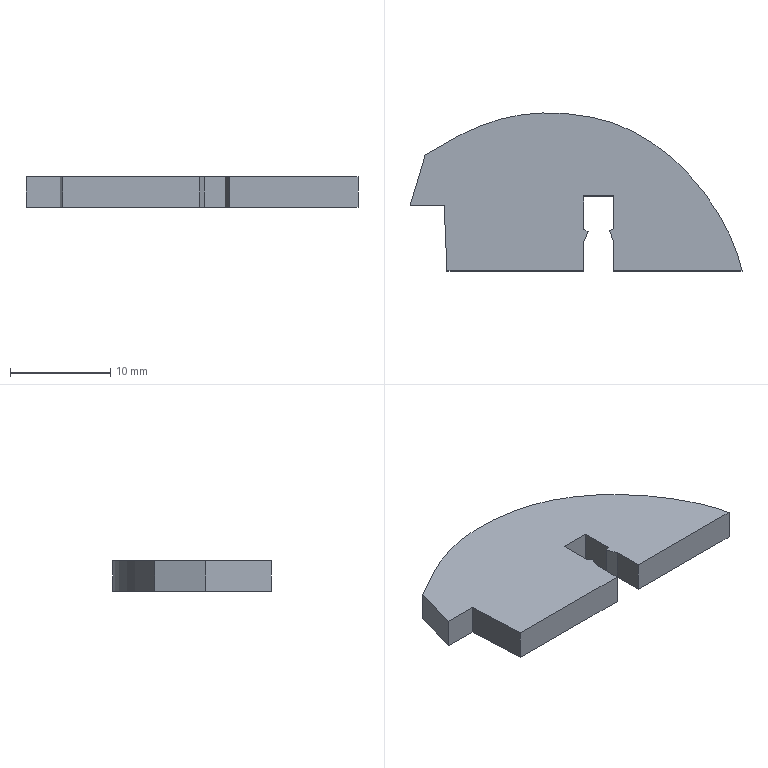Part | SolidWorks | features BaseBody 1 | 1 solid | 18 faces | box 33.145 x 15.784 x 3 mm | volume 1116 mm3 | plane 15 | spline 3
STEP:
#1=CARTESIAN_POINT('',(-1.198,15.692,-1.5));
#2=VERTEX_POINT('',#1);
#3=CARTESIAN_POINT('',(13.751,0.3596,-1.5));
#4=VERTEX_POINT('',#3);
#5=CARTESIAN_POINT('',(-1.198,15.692,-1.5));
#6=CARTESIAN_POINT('',(7.041,14.092,-1.5));
#7=CARTESIAN_POINT('',(12.666,5.726,-1.5));
#8=CARTESIAN_POINT('',(13.751,0.3596,-1.5));
#9=B_SPLINE_CURVE_WITH_KNOTS('',3,(#5,#6,#7,#8),.UNSPECIFIED.,.F.,.F.,(4,4),(0.3636,0.4545),.UNSPECIFIED.);
#10=EDGE_CURVE('',#2,#4,#9,.T.);
#11=ORIENTED_EDGE('',*,*,#10,.T.);
#12=CARTESIAN_POINT('',(0.9453,0.3596,-1.5));
#13=VERTEX_POINT('',#12);
#14=CARTESIAN_POINT('',(0.,0.3596,-1.5));
#15=DIRECTION('',(-1.,0.,0.));
#16=VECTOR('',#15,1000.);
#17=LINE('',#14,#16);
#18=EDGE_CURVE('',#4,#13,#17,.T.);
#19=ORIENTED_EDGE('',*,*,#18,.T.);
#20=CARTESIAN_POINT('',(0.9453,3.34,-1.5));
#21=VERTEX_POINT('',#20);
#22=CARTESIAN_POINT('',(0.9453,0.,-1.5));
#23=DIRECTION('',(0.,-1.,0.));
#24=VECTOR('',#23,1000.);
#25=LINE('',#22,#24);
#26=EDGE_CURVE('',#21,#13,#25,.T.);
#27=ORIENTED_EDGE('',*,*,#26,.F.);
#28=CARTESIAN_POINT('',(0.4951,4.381,-1.5));
#29=VERTEX_POINT('',#28);
#30=CARTESIAN_POINT('',(2.013,0.8704,-1.5));
#31=DIRECTION('',(0.3969,-0.9179,0.));
#32=VECTOR('',#31,1000.);
#33=LINE('',#30,#32);
#34=EDGE_CURVE('',#29,#21,#33,.T.);
#35=ORIENTED_EDGE('',*,*,#34,.F.);
#36=CARTESIAN_POINT('',(0.9453,4.577,-1.5));
#37=VERTEX_POINT('',#36);
#38=CARTESIAN_POINT('',(-1.524,3.502,-1.5));
#39=DIRECTION('',(-0.9169,-0.3992,0.));
#40=VECTOR('',#39,1000.);
#41=LINE('',#38,#40);
#42=EDGE_CURVE('',#37,#29,#41,.T.);
#43=ORIENTED_EDGE('',*,*,#42,.F.);
#44=CARTESIAN_POINT('',(0.9453,7.848,-1.5));
#45=VERTEX_POINT('',#44);
#46=CARTESIAN_POINT('',(0.9453,0.,-1.5));
#47=DIRECTION('',(0.,-1.,0.));
#48=VECTOR('',#47,1000.);
#49=LINE('',#46,#48);
#50=EDGE_CURVE('',#45,#37,#49,.T.);
#51=ORIENTED_EDGE('',*,*,#50,.F.);
#52=CARTESIAN_POINT('',(-2.051,7.848,-1.5));
#53=VERTEX_POINT('',#52);
#54=CARTESIAN_POINT('',(0.,7.848,-1.5));
#55=DIRECTION('',(1.,0.,0.));
#56=VECTOR('',#55,1000.);
#57=LINE('',#54,#56);
#58=EDGE_CURVE('',#53,#45,#57,.T.);
#59=ORIENTED_EDGE('',*,*,#58,.F.);
#60=CARTESIAN_POINT('',(-2.051,4.544,-1.5));
#61=VERTEX_POINT('',#60);
#62=CARTESIAN_POINT('',(-2.051,0.,-1.5));
#63=DIRECTION('',(0.,1.,0.));
#64=VECTOR('',#63,1000.);
#65=LINE('',#62,#64);
#66=EDGE_CURVE('',#61,#53,#65,.T.);
#67=ORIENTED_EDGE('',*,*,#66,.F.);
#68=CARTESIAN_POINT('',(-1.602,4.279,-1.5));
#69=VERTEX_POINT('',#68);
#70=CARTESIAN_POINT('',(1.459,2.47,-1.5));
#71=DIRECTION('',(-0.861,0.5086,0.));
#72=VECTOR('',#71,1000.);
#73=LINE('',#70,#72);
#74=EDGE_CURVE('',#69,#61,#73,.T.);
#75=ORIENTED_EDGE('',*,*,#74,.F.);
#76=CARTESIAN_POINT('',(-2.051,3.321,-1.5));
#77=VERTEX_POINT('',#76);
#78=CARTESIAN_POINT('',(-2.957,1.385,-1.5));
#79=DIRECTION('',(0.4242,0.9056,0.));
#80=VECTOR('',#79,1000.);
#81=LINE('',#78,#80);
#82=EDGE_CURVE('',#77,#69,#81,.T.);
#83=ORIENTED_EDGE('',*,*,#82,.F.);
#84=CARTESIAN_POINT('',(-2.051,0.3596,-1.5));
#85=VERTEX_POINT('',#84);
#86=CARTESIAN_POINT('',(-2.051,0.,-1.5));
#87=DIRECTION('',(0.,1.,0.));
#88=VECTOR('',#87,1000.);
#89=LINE('',#86,#88);
#90=EDGE_CURVE('',#85,#77,#89,.T.);
#91=ORIENTED_EDGE('',*,*,#90,.F.);
#92=CARTESIAN_POINT('',(-15.701,0.3596,-1.5));
#93=VERTEX_POINT('',#92);
#94=CARTESIAN_POINT('',(0.,0.3596,-1.5));
#95=DIRECTION('',(-1.,0.,0.));
#96=VECTOR('',#95,1000.);
#97=LINE('',#94,#96);
#98=EDGE_CURVE('',#85,#93,#97,.T.);
#99=ORIENTED_EDGE('',*,*,#98,.T.);
#100=CARTESIAN_POINT('',(-15.986,6.867,-1.5));
#101=VERTEX_POINT('',#100);
#102=CARTESIAN_POINT('',(-15.701,0.3596,-1.5));
#103=CARTESIAN_POINT('',(-15.797,2.531,-1.5));
#104=CARTESIAN_POINT('',(-15.89,4.698,-1.5));
#105=CARTESIAN_POINT('',(-15.986,6.867,-1.5));
#106=B_SPLINE_CURVE_WITH_KNOTS('',3,(#102,#103,#104,#105),.UNSPECIFIED.,.F.,.F.,(4,4),(0.,0.09091),.UNSPECIFIED.);
#107=EDGE_CURVE('',#93,#101,#106,.T.);
#108=ORIENTED_EDGE('',*,*,#107,.T.);
#109=CARTESIAN_POINT('',(-19.394,6.867,-1.5));
#110=VERTEX_POINT('',#109);
#111=CARTESIAN_POINT('',(0.,6.867,-1.5));
#112=DIRECTION('',(-1.,0.,0.));
#113=VECTOR('',#112,1000.);
#114=LINE('',#111,#113);
#115=EDGE_CURVE('',#101,#110,#114,.T.);
#116=ORIENTED_EDGE('',*,*,#115,.T.);
#117=CARTESIAN_POINT('',(-17.871,11.949,-1.5));
#118=VERTEX_POINT('',#117);
#119=CARTESIAN_POINT('',(-19.684,5.899,-1.5));
#120=DIRECTION('',(0.2871,0.9579,0.));
#121=VECTOR('',#120,1000.);
#122=LINE('',#119,#121);
#123=EDGE_CURVE('',#110,#118,#122,.T.);
#124=ORIENTED_EDGE('',*,*,#123,.T.);
#125=CARTESIAN_POINT('',(-17.871,11.949,-1.5));
#126=CARTESIAN_POINT('',(-13.479,14.586,-1.5));
#127=CARTESIAN_POINT('',(-9.088,17.223,-1.5));
#128=CARTESIAN_POINT('',(-1.198,15.692,-1.5));
#129=B_SPLINE_CURVE_WITH_KNOTS('',3,(#125,#126,#127,#128),.UNSPECIFIED.,.F.,.F.,(4,4),(0.2727,0.3636),.UNSPECIFIED.);
#130=EDGE_CURVE('',#118,#2,#129,.T.);
#131=ORIENTED_EDGE('',*,*,#130,.T.);
#132=EDGE_LOOP('',(#11,#19,#27,#35,#43,#51,#59,#67,#75,#83,#91,#99,#108,#116,#124,#131));
#133=FACE_OUTER_BOUND('',#132,.T.);
#134=CARTESIAN_POINT('',(0.,0.,-1.5));
#135=DIRECTION('',(0.,0.,1.));
#136=DIRECTION('',(1.,0.,0.));
#137=AXIS2_PLACEMENT_3D('',#134,#135,#136);
#138=PLANE('',#137);
#139=ADVANCED_FACE('',(#133),#138,.F.);
#140=CARTESIAN_POINT('',(-1.198,15.692,1.5));
#141=VERTEX_POINT('',#140);
#142=CARTESIAN_POINT('',(13.751,0.3596,1.5));
#143=VERTEX_POINT('',#142);
#144=CARTESIAN_POINT('',(-1.198,15.692,1.5));
#145=CARTESIAN_POINT('',(7.041,14.092,1.5));
#146=CARTESIAN_POINT('',(12.666,5.726,1.5));
#147=CARTESIAN_POINT('',(13.751,0.3596,1.5));
#148=B_SPLINE_CURVE_WITH_KNOTS('',3,(#144,#145,#146,#147),.UNSPECIFIED.,.F.,.F.,(4,4),(0.3636,0.4545),.UNSPECIFIED.);
#149=EDGE_CURVE('',#141,#143,#148,.T.);
#150=ORIENTED_EDGE('',*,*,#149,.F.);
#151=CARTESIAN_POINT('',(-17.871,11.949,1.5));
#152=VERTEX_POINT('',#151);
#153=CARTESIAN_POINT('',(-17.871,11.949,1.5));
#154=CARTESIAN_POINT('',(-13.479,14.586,1.5));
#155=CARTESIAN_POINT('',(-9.088,17.223,1.5));
#156=CARTESIAN_POINT('',(-1.198,15.692,1.5));
#157=B_SPLINE_CURVE_WITH_KNOTS('',3,(#153,#154,#155,#156),.UNSPECIFIED.,.F.,.F.,(4,4),(0.2727,0.3636),.UNSPECIFIED.);
#158=EDGE_CURVE('',#152,#141,#157,.T.);
#159=ORIENTED_EDGE('',*,*,#158,.F.);
#160=CARTESIAN_POINT('',(-19.394,6.867,1.5));
#161=VERTEX_POINT('',#160);
#162=CARTESIAN_POINT('',(-19.684,5.899,1.5));
#163=DIRECTION('',(0.2871,0.9579,0.));
#164=VECTOR('',#163,1000.);
#165=LINE('',#162,#164);
#166=EDGE_CURVE('',#161,#152,#165,.T.);
#167=ORIENTED_EDGE('',*,*,#166,.F.);
#168=CARTESIAN_POINT('',(-15.986,6.867,1.5));
#169=VERTEX_POINT('',#168);
#170=CARTESIAN_POINT('',(0.,6.867,1.5));
#171=DIRECTION('',(-1.,0.,0.));
#172=VECTOR('',#171,1000.);
#173=LINE('',#170,#172);
#174=EDGE_CURVE('',#169,#161,#173,.T.);
#175=ORIENTED_EDGE('',*,*,#174,.F.);
#176=CARTESIAN_POINT('',(-15.701,0.3596,1.5));
#177=VERTEX_POINT('',#176);
#178=CARTESIAN_POINT('',(-15.701,0.3596,1.5));
#179=CARTESIAN_POINT('',(-15.797,2.531,1.5));
#180=CARTESIAN_POINT('',(-15.89,4.698,1.5));
#181=CARTESIAN_POINT('',(-15.986,6.867,1.5));
#182=B_SPLINE_CURVE_WITH_KNOTS('',3,(#178,#179,#180,#181),.UNSPECIFIED.,.F.,.F.,(4,4),(0.,0.09091),.UNSPECIFIED.);
#183=EDGE_CURVE('',#177,#169,#182,.T.);
#184=ORIENTED_EDGE('',*,*,#183,.F.);
#185=CARTESIAN_POINT('',(-2.051,0.3596,1.5));
#186=VERTEX_POINT('',#185);
#187=CARTESIAN_POINT('',(0.,0.3596,1.5));
#188=DIRECTION('',(-1.,0.,0.));
#189=VECTOR('',#188,1000.);
#190=LINE('',#187,#189);
#191=EDGE_CURVE('',#186,#177,#190,.T.);
#192=ORIENTED_EDGE('',*,*,#191,.F.);
#193=CARTESIAN_POINT('',(-2.051,3.321,1.5));
#194=VERTEX_POINT('',#193);
#195=CARTESIAN_POINT('',(-2.051,0.,1.5));
#196=DIRECTION('',(0.,1.,0.));
#197=VECTOR('',#196,1000.);
#198=LINE('',#195,#197);
#199=EDGE_CURVE('',#186,#194,#198,.T.);
#200=ORIENTED_EDGE('',*,*,#199,.T.);
#201=CARTESIAN_POINT('',(-1.602,4.279,1.5));
#202=VERTEX_POINT('',#201);
#203=CARTESIAN_POINT('',(-2.957,1.385,1.5));
#204=DIRECTION('',(0.4242,0.9056,0.));
#205=VECTOR('',#204,1000.);
#206=LINE('',#203,#205);
#207=EDGE_CURVE('',#194,#202,#206,.T.);
#208=ORIENTED_EDGE('',*,*,#207,.T.);
#209=CARTESIAN_POINT('',(-2.051,4.544,1.5));
#210=VERTEX_POINT('',#209);
#211=CARTESIAN_POINT('',(1.459,2.47,1.5));
#212=DIRECTION('',(-0.861,0.5086,0.));
#213=VECTOR('',#212,1000.);
#214=LINE('',#211,#213);
#215=EDGE_CURVE('',#202,#210,#214,.T.);
#216=ORIENTED_EDGE('',*,*,#215,.T.);
#217=CARTESIAN_POINT('',(-2.051,7.848,1.5));
#218=VERTEX_POINT('',#217);
#219=CARTESIAN_POINT('',(-2.051,0.,1.5));
#220=DIRECTION('',(0.,1.,0.));
#221=VECTOR('',#220,1000.);
#222=LINE('',#219,#221);
#223=EDGE_CURVE('',#210,#218,#222,.T.);
#224=ORIENTED_EDGE('',*,*,#223,.T.);
#225=CARTESIAN_POINT('',(0.9453,7.848,1.5));
#226=VERTEX_POINT('',#225);
#227=CARTESIAN_POINT('',(0.,7.848,1.5));
#228=DIRECTION('',(1.,0.,0.));
#229=VECTOR('',#228,1000.);
#230=LINE('',#227,#229);
#231=EDGE_CURVE('',#218,#226,#230,.T.);
#232=ORIENTED_EDGE('',*,*,#231,.T.);
#233=CARTESIAN_POINT('',(0.9453,4.577,1.5));
#234=VERTEX_POINT('',#233);
#235=CARTESIAN_POINT('',(0.9453,0.,1.5));
#236=DIRECTION('',(0.,-1.,0.));
#237=VECTOR('',#236,1000.);
#238=LINE('',#235,#237);
#239=EDGE_CURVE('',#226,#234,#238,.T.);
#240=ORIENTED_EDGE('',*,*,#239,.T.);
#241=CARTESIAN_POINT('',(0.4951,4.381,1.5));
#242=VERTEX_POINT('',#241);
#243=CARTESIAN_POINT('',(-1.524,3.502,1.5));
#244=DIRECTION('',(-0.9169,-0.3992,0.));
#245=VECTOR('',#244,1000.);
#246=LINE('',#243,#245);
#247=EDGE_CURVE('',#234,#242,#246,.T.);
#248=ORIENTED_EDGE('',*,*,#247,.T.);
#249=CARTESIAN_POINT('',(0.9453,3.34,1.5));
#250=VERTEX_POINT('',#249);
#251=CARTESIAN_POINT('',(2.013,0.8704,1.5));
#252=DIRECTION('',(0.3969,-0.9179,0.));
#253=VECTOR('',#252,1000.);
#254=LINE('',#251,#253);
#255=EDGE_CURVE('',#242,#250,#254,.T.);
#256=ORIENTED_EDGE('',*,*,#255,.T.);
#257=CARTESIAN_POINT('',(0.9453,0.3596,1.5));
#258=VERTEX_POINT('',#257);
#259=CARTESIAN_POINT('',(0.9453,0.,1.5));
#260=DIRECTION('',(0.,-1.,0.));
#261=VECTOR('',#260,1000.);
#262=LINE('',#259,#261);
#263=EDGE_CURVE('',#250,#258,#262,.T.);
#264=ORIENTED_EDGE('',*,*,#263,.T.);
#265=CARTESIAN_POINT('',(0.,0.3596,1.5));
#266=DIRECTION('',(-1.,0.,0.));
#267=VECTOR('',#266,1000.);
#268=LINE('',#265,#267);
#269=EDGE_CURVE('',#143,#258,#268,.T.);
#270=ORIENTED_EDGE('',*,*,#269,.F.);
#271=EDGE_LOOP('',(#150,#159,#167,#175,#184,#192,#200,#208,#216,#224,#232,#240,#248,#256,#264,#270));
#272=FACE_OUTER_BOUND('',#271,.T.);
#273=CARTESIAN_POINT('',(0.,0.,1.5));
#274=DIRECTION('',(0.,0.,1.));
#275=DIRECTION('',(1.,0.,0.));
#276=AXIS2_PLACEMENT_3D('',#273,#274,#275);
#277=PLANE('',#276);
#278=ADVANCED_FACE('',(#272),#277,.T.);
#279=ORIENTED_EDGE('',*,*,#18,.F.);
#280=CARTESIAN_POINT('',(13.751,0.3596,1.5));
#281=DIRECTION('',(0.,0.,-1.));
#282=VECTOR('',#281,1000.);
#283=LINE('',#280,#282);
#284=EDGE_CURVE('',#143,#4,#283,.T.);
#285=ORIENTED_EDGE('',*,*,#284,.F.);
#286=ORIENTED_EDGE('',*,*,#269,.T.);
#287=CARTESIAN_POINT('',(0.9453,0.3596,1.5));
#288=DIRECTION('',(0.,0.,-1.));
#289=VECTOR('',#288,1000.);
#290=LINE('',#287,#289);
#291=EDGE_CURVE('',#258,#13,#290,.T.);
#292=ORIENTED_EDGE('',*,*,#291,.T.);
#293=EDGE_LOOP('',(#279,#285,#286,#292));
#294=FACE_OUTER_BOUND('',#293,.T.);
#295=CARTESIAN_POINT('',(0.,0.3596,1.5));
#296=DIRECTION('',(0.,-1.,0.));
#297=DIRECTION('',(0.,0.,-1.));
#298=AXIS2_PLACEMENT_3D('',#295,#296,#297);
#299=PLANE('',#298);
#300=ADVANCED_FACE('',(#294),#299,.T.);
#301=ORIENTED_EDGE('',*,*,#26,.T.);
#302=ORIENTED_EDGE('',*,*,#291,.F.);
#303=ORIENTED_EDGE('',*,*,#263,.F.);
#304=CARTESIAN_POINT('',(0.9453,3.34,1.5));
#305=DIRECTION('',(0.,0.,-1.));
#306=VECTOR('',#305,1000.);
#307=LINE('',#304,#306);
#308=EDGE_CURVE('',#250,#21,#307,.T.);
#309=ORIENTED_EDGE('',*,*,#308,.T.);
#310=EDGE_LOOP('',(#301,#302,#303,#309));
#311=FACE_OUTER_BOUND('',#310,.T.);
#312=CARTESIAN_POINT('',(0.9453,0.,1.5));
#313=DIRECTION('',(1.,0.,0.));
#314=DIRECTION('',(0.,1.,0.));
#315=AXIS2_PLACEMENT_3D('',#312,#313,#314);
#316=PLANE('',#315);
#317=ADVANCED_FACE('',(#311),#316,.F.);
#318=ORIENTED_EDGE('',*,*,#34,.T.);
#319=ORIENTED_EDGE('',*,*,#308,.F.);
#320=ORIENTED_EDGE('',*,*,#255,.F.);
#321=CARTESIAN_POINT('',(0.4951,4.381,1.5));
#322=DIRECTION('',(0.,0.,-1.));
#323=VECTOR('',#322,1000.);
#324=LINE('',#321,#323);
#325=EDGE_CURVE('',#242,#29,#324,.T.);
#326=ORIENTED_EDGE('',*,*,#325,.T.);
#327=EDGE_LOOP('',(#318,#319,#320,#326));
#328=FACE_OUTER_BOUND('',#327,.T.);
#329=CARTESIAN_POINT('',(2.013,0.8704,1.5));
#330=DIRECTION('',(0.9179,0.3969,0.));
#331=DIRECTION('',(0.,0.,-1.));
#332=AXIS2_PLACEMENT_3D('',#329,#330,#331);
#333=PLANE('',#332);
#334=ADVANCED_FACE('',(#328),#333,.F.);
#335=ORIENTED_EDGE('',*,*,#42,.T.);
#336=ORIENTED_EDGE('',*,*,#325,.F.);
#337=ORIENTED_EDGE('',*,*,#247,.F.);
#338=CARTESIAN_POINT('',(0.9453,4.577,1.5));
#339=DIRECTION('',(0.,0.,-1.));
#340=VECTOR('',#339,1000.);
#341=LINE('',#338,#340);
#342=EDGE_CURVE('',#234,#37,#341,.T.);
#343=ORIENTED_EDGE('',*,*,#342,.T.);
#344=EDGE_LOOP('',(#335,#336,#337,#343));
#345=FACE_OUTER_BOUND('',#344,.T.);
#346=CARTESIAN_POINT('',(-1.524,3.502,1.5));
#347=DIRECTION('',(0.3992,-0.9169,0.));
#348=DIRECTION('',(0.,0.,-1.));
#349=AXIS2_PLACEMENT_3D('',#346,#347,#348);
#350=PLANE('',#349);
#351=ADVANCED_FACE('',(#345),#350,.F.);
#352=ORIENTED_EDGE('',*,*,#50,.T.);
#353=ORIENTED_EDGE('',*,*,#342,.F.);
#354=ORIENTED_EDGE('',*,*,#239,.F.);
#355=CARTESIAN_POINT('',(0.9453,7.848,1.5));
#356=DIRECTION('',(0.,0.,-1.));
#357=VECTOR('',#356,1000.);
#358=LINE('',#355,#357);
#359=EDGE_CURVE('',#226,#45,#358,.T.);
#360=ORIENTED_EDGE('',*,*,#359,.T.);
#361=EDGE_LOOP('',(#352,#353,#354,#360));
#362=FACE_OUTER_BOUND('',#361,.T.);
#363=CARTESIAN_POINT('',(0.9453,0.,1.5));
#364=DIRECTION('',(1.,0.,0.));
#365=DIRECTION('',(0.,1.,0.));
#366=AXIS2_PLACEMENT_3D('',#363,#364,#365);
#367=PLANE('',#366);
#368=ADVANCED_FACE('',(#362),#367,.F.);
#369=ORIENTED_EDGE('',*,*,#58,.T.);
#370=ORIENTED_EDGE('',*,*,#359,.F.);
#371=ORIENTED_EDGE('',*,*,#231,.F.);
#372=CARTESIAN_POINT('',(-2.051,7.848,1.5));
#373=DIRECTION('',(0.,0.,-1.));
#374=VECTOR('',#373,1000.);
#375=LINE('',#372,#374);
#376=EDGE_CURVE('',#218,#53,#375,.T.);
#377=ORIENTED_EDGE('',*,*,#376,.T.);
#378=EDGE_LOOP('',(#369,#370,#371,#377));
#379=FACE_OUTER_BOUND('',#378,.T.);
#380=CARTESIAN_POINT('',(0.,7.848,1.5));
#381=DIRECTION('',(0.,1.,0.));
#382=DIRECTION('',(1.,0.,0.));
#383=AXIS2_PLACEMENT_3D('',#380,#381,#382);
#384=PLANE('',#383);
#385=ADVANCED_FACE('',(#379),#384,.F.);
#386=ORIENTED_EDGE('',*,*,#66,.T.);
#387=ORIENTED_EDGE('',*,*,#376,.F.);
#388=ORIENTED_EDGE('',*,*,#223,.F.);
#389=CARTESIAN_POINT('',(-2.051,4.544,1.5));
#390=DIRECTION('',(0.,0.,-1.));
#391=VECTOR('',#390,1000.);
#392=LINE('',#389,#391);
#393=EDGE_CURVE('',#210,#61,#392,.T.);
#394=ORIENTED_EDGE('',*,*,#393,.T.);
#395=EDGE_LOOP('',(#386,#387,#388,#394));
#396=FACE_OUTER_BOUND('',#395,.T.);
#397=CARTESIAN_POINT('',(-2.051,0.,1.5));
#398=DIRECTION('',(-1.,0.,0.));
#399=DIRECTION('',(0.,0.,1.));
#400=AXIS2_PLACEMENT_3D('',#397,#398,#399);
#401=PLANE('',#400);
#402=ADVANCED_FACE('',(#396),#401,.F.);
#403=ORIENTED_EDGE('',*,*,#74,.T.);
#404=ORIENTED_EDGE('',*,*,#393,.F.);
#405=ORIENTED_EDGE('',*,*,#215,.F.);
#406=CARTESIAN_POINT('',(-1.602,4.279,1.5));
#407=DIRECTION('',(0.,0.,-1.));
#408=VECTOR('',#407,1000.);
#409=LINE('',#406,#408);
#410=EDGE_CURVE('',#202,#69,#409,.T.);
#411=ORIENTED_EDGE('',*,*,#410,.T.);
#412=EDGE_LOOP('',(#403,#404,#405,#411));
#413=FACE_OUTER_BOUND('',#412,.T.);
#414=CARTESIAN_POINT('',(1.459,2.47,1.5));
#415=DIRECTION('',(-0.5086,-0.861,0.));
#416=DIRECTION('',(-0.861,0.5086,0.));
#417=AXIS2_PLACEMENT_3D('',#414,#415,#416);
#418=PLANE('',#417);
#419=ADVANCED_FACE('',(#413),#418,.F.);
#420=ORIENTED_EDGE('',*,*,#82,.T.);
#421=ORIENTED_EDGE('',*,*,#410,.F.);
#422=ORIENTED_EDGE('',*,*,#207,.F.);
#423=CARTESIAN_POINT('',(-2.051,3.321,1.5));
#424=DIRECTION('',(0.,0.,-1.));
#425=VECTOR('',#424,1000.);
#426=LINE('',#423,#425);
#427=EDGE_CURVE('',#194,#77,#426,.T.);
#428=ORIENTED_EDGE('',*,*,#427,.T.);
#429=EDGE_LOOP('',(#420,#421,#422,#428));
#430=FACE_OUTER_BOUND('',#429,.T.);
#431=CARTESIAN_POINT('',(-2.957,1.385,1.5));
#432=DIRECTION('',(-0.9056,0.4242,0.));
#433=DIRECTION('',(0.,0.,1.));
#434=AXIS2_PLACEMENT_3D('',#431,#432,#433);
#435=PLANE('',#434);
#436=ADVANCED_FACE('',(#430),#435,.F.);
#437=ORIENTED_EDGE('',*,*,#90,.T.);
#438=ORIENTED_EDGE('',*,*,#427,.F.);
#439=ORIENTED_EDGE('',*,*,#199,.F.);
#440=CARTESIAN_POINT('',(-2.051,0.3596,1.5));
#441=DIRECTION('',(0.,0.,-1.));
#442=VECTOR('',#441,1000.);
#443=LINE('',#440,#442);
#444=EDGE_CURVE('',#186,#85,#443,.T.);
#445=ORIENTED_EDGE('',*,*,#444,.T.);
#446=EDGE_LOOP('',(#437,#438,#439,#445));
#447=FACE_OUTER_BOUND('',#446,.T.);
#448=CARTESIAN_POINT('',(-2.051,0.,1.5));
#449=DIRECTION('',(-1.,0.,0.));
#450=DIRECTION('',(0.,0.,1.));
#451=AXIS2_PLACEMENT_3D('',#448,#449,#450);
#452=PLANE('',#451);
#453=ADVANCED_FACE('',(#447),#452,.F.);
#454=ORIENTED_EDGE('',*,*,#98,.F.);
#455=ORIENTED_EDGE('',*,*,#444,.F.);
#456=ORIENTED_EDGE('',*,*,#191,.T.);
#457=CARTESIAN_POINT('',(-15.701,0.3596,1.5));
#458=DIRECTION('',(0.,0.,-1.));
#459=VECTOR('',#458,1000.);
#460=LINE('',#457,#459);
#461=EDGE_CURVE('',#177,#93,#460,.T.);
#462=ORIENTED_EDGE('',*,*,#461,.T.);
#463=EDGE_LOOP('',(#454,#455,#456,#462));
#464=FACE_OUTER_BOUND('',#463,.T.);
#465=CARTESIAN_POINT('',(0.,0.3596,1.5));
#466=DIRECTION('',(0.,-1.,0.));
#467=DIRECTION('',(0.,0.,-1.));
#468=AXIS2_PLACEMENT_3D('',#465,#466,#467);
#469=PLANE('',#468);
#470=ADVANCED_FACE('',(#464),#469,.T.);
#471=ORIENTED_EDGE('',*,*,#107,.F.);
#472=ORIENTED_EDGE('',*,*,#461,.F.);
#473=ORIENTED_EDGE('',*,*,#183,.T.);
#474=CARTESIAN_POINT('',(-15.986,6.867,1.5));
#475=DIRECTION('',(0.,0.,-1.));
#476=VECTOR('',#475,1000.);
#477=LINE('',#474,#476);
#478=EDGE_CURVE('',#169,#101,#477,.T.);
#479=ORIENTED_EDGE('',*,*,#478,.T.);
#480=EDGE_LOOP('',(#471,#472,#473,#479));
#481=FACE_OUTER_BOUND('',#480,.T.);
#482=CARTESIAN_POINT('',(-15.701,0.3596,1.5));
#483=CARTESIAN_POINT('',(-15.701,0.3596,-1.5));
#484=CARTESIAN_POINT('',(-15.797,2.531,1.5));
#485=CARTESIAN_POINT('',(-15.797,2.531,-1.5));
#486=CARTESIAN_POINT('',(-15.89,4.698,1.5));
#487=CARTESIAN_POINT('',(-15.89,4.698,-1.5));
#488=CARTESIAN_POINT('',(-15.986,6.867,1.5));
#489=CARTESIAN_POINT('',(-15.986,6.867,-1.5));
#490=B_SPLINE_SURFACE_WITH_KNOTS('',3,1,((#482,#483),(#484,#485),(#486,#487),(#488,#489)),.UNSPECIFIED.,.F.,.F.,.F.,(4,4),(2,2),(0.,0.09091),(0.,1.),.UNSPECIFIED.);
#491=ADVANCED_FACE('',(#481),#490,.T.);
#492=ORIENTED_EDGE('',*,*,#115,.F.);
#493=ORIENTED_EDGE('',*,*,#478,.F.);
#494=ORIENTED_EDGE('',*,*,#174,.T.);
#495=CARTESIAN_POINT('',(-19.394,6.867,1.5));
#496=DIRECTION('',(0.,0.,-1.));
#497=VECTOR('',#496,1000.);
#498=LINE('',#495,#497);
#499=EDGE_CURVE('',#161,#110,#498,.T.);
#500=ORIENTED_EDGE('',*,*,#499,.T.);
#501=EDGE_LOOP('',(#492,#493,#494,#500));
#502=FACE_OUTER_BOUND('',#501,.T.);
#503=CARTESIAN_POINT('',(0.,6.867,1.5));
#504=DIRECTION('',(0.,-1.,0.));
#505=DIRECTION('',(0.,0.,-1.));
#506=AXIS2_PLACEMENT_3D('',#503,#504,#505);
#507=PLANE('',#506);
#508=ADVANCED_FACE('',(#502),#507,.T.);
#509=ORIENTED_EDGE('',*,*,#123,.F.);
#510=ORIENTED_EDGE('',*,*,#499,.F.);
#511=ORIENTED_EDGE('',*,*,#166,.T.);
#512=CARTESIAN_POINT('',(-17.871,11.949,1.5));
#513=DIRECTION('',(0.,0.,-1.));
#514=VECTOR('',#513,1000.);
#515=LINE('',#512,#514);
#516=EDGE_CURVE('',#152,#118,#515,.T.);
#517=ORIENTED_EDGE('',*,*,#516,.T.);
#518=EDGE_LOOP('',(#509,#510,#511,#517));
#519=FACE_OUTER_BOUND('',#518,.T.);
#520=CARTESIAN_POINT('',(-19.684,5.899,1.5));
#521=DIRECTION('',(-0.9579,0.2871,0.));
#522=DIRECTION('',(0.,0.,1.));
#523=AXIS2_PLACEMENT_3D('',#520,#521,#522);
#524=PLANE('',#523);
#525=ADVANCED_FACE('',(#519),#524,.T.);
#526=ORIENTED_EDGE('',*,*,#130,.F.);
#527=ORIENTED_EDGE('',*,*,#516,.F.);
#528=ORIENTED_EDGE('',*,*,#158,.T.);
#529=CARTESIAN_POINT('',(-1.198,15.692,1.5));
#530=DIRECTION('',(0.,0.,-1.));
#531=VECTOR('',#530,1000.);
#532=LINE('',#529,#531);
#533=EDGE_CURVE('',#141,#2,#532,.T.);
#534=ORIENTED_EDGE('',*,*,#533,.T.);
#535=EDGE_LOOP('',(#526,#527,#528,#534));
#536=FACE_OUTER_BOUND('',#535,.T.);
#537=CARTESIAN_POINT('',(-17.871,11.949,1.5));
#538=CARTESIAN_POINT('',(-17.871,11.949,-1.5));
#539=CARTESIAN_POINT('',(-13.479,14.586,1.5));
#540=CARTESIAN_POINT('',(-13.479,14.586,-1.5));
#541=CARTESIAN_POINT('',(-9.088,17.223,1.5));
#542=CARTESIAN_POINT('',(-9.088,17.223,-1.5));
#543=CARTESIAN_POINT('',(-1.198,15.692,1.5));
#544=CARTESIAN_POINT('',(-1.198,15.692,-1.5));
#545=B_SPLINE_SURFACE_WITH_KNOTS('',3,1,((#537,#538),(#539,#540),(#541,#542),(#543,#544)),.UNSPECIFIED.,.F.,.F.,.F.,(4,4),(2,2),(0.2727,0.3636),(0.,1.),.UNSPECIFIED.);
#546=ADVANCED_FACE('',(#536),#545,.T.);
#547=ORIENTED_EDGE('',*,*,#10,.F.);
#548=ORIENTED_EDGE('',*,*,#533,.F.);
#549=ORIENTED_EDGE('',*,*,#149,.T.);
#550=ORIENTED_EDGE('',*,*,#284,.T.);
#551=EDGE_LOOP('',(#547,#548,#549,#550));
#552=FACE_OUTER_BOUND('',#551,.T.);
#553=CARTESIAN_POINT('',(-1.198,15.692,1.5));
#554=CARTESIAN_POINT('',(-1.198,15.692,-1.5));
#555=CARTESIAN_POINT('',(7.041,14.092,1.5));
#556=CARTESIAN_POINT('',(7.041,14.092,-1.5));
#557=CARTESIAN_POINT('',(12.666,5.726,1.5));
#558=CARTESIAN_POINT('',(12.666,5.726,-1.5));
#559=CARTESIAN_POINT('',(13.751,0.3596,1.5));
#560=CARTESIAN_POINT('',(13.751,0.3596,-1.5));
#561=B_SPLINE_SURFACE_WITH_KNOTS('',3,1,((#553,#554),(#555,#556),(#557,#558),(#559,#560)),.UNSPECIFIED.,.F.,.F.,.F.,(4,4),(2,2),(0.3636,0.4545),(0.,1.),.UNSPECIFIED.);
#562=ADVANCED_FACE('',(#552),#561,.T.);
#563=CLOSED_SHELL('',(#139,#278,#300,#317,#334,#351,#368,#385,#402,#419,#436,#453,#470,#491,#508,#525,#546,#562));
#564=MANIFOLD_SOLID_BREP('',#563);
#565=CARTESIAN_POINT('',(0.,0.,0.));
#566=DIRECTION('',(0.,0.,1.));
#567=DIRECTION('',(1.,0.,0.));
#568=AXIS2_PLACEMENT_3D('',#565,#566,#567);
#569=(LENGTH_UNIT()NAMED_UNIT(*)SI_UNIT(.MILLI.,.METRE.));
#570=UNCERTAINTY_MEASURE_WITH_UNIT(LENGTH_MEASURE(0.00001),#569,'','');
#571=(NAMED_UNIT(*)PLANE_ANGLE_UNIT()SI_UNIT($,.RADIAN.));
#572=(NAMED_UNIT(*)SI_UNIT($,.STERADIAN.)SOLID_ANGLE_UNIT());
#573=(GEOMETRIC_REPRESENTATION_CONTEXT(3)GLOBAL_UNCERTAINTY_ASSIGNED_CONTEXT((#570))GLOBAL_UNIT_ASSIGNED_CONTEXT((#569,#571,#572))REPRESENTATION_CONTEXT('',''));
#574=ADVANCED_BREP_SHAPE_REPRESENTATION('',(#564,#568),#573);